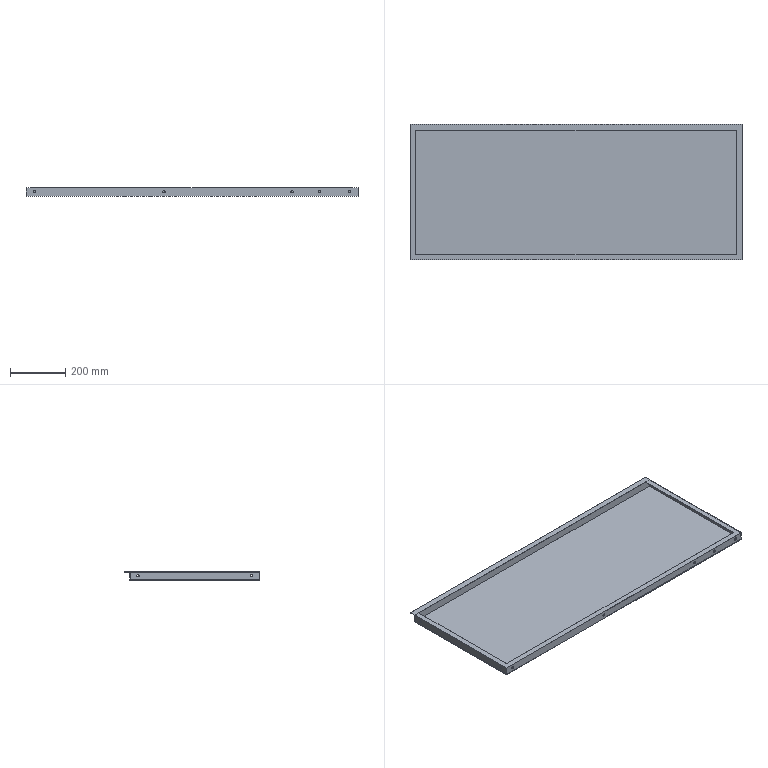Part | SolidWorks | features ICE 3, Extrusion 1, Shell 1 | 1 solid | 35 faces | box 1204 x 492 x 30 mm | volume 1446455 mm3 | cylinder 18 | plane 17 | commonest cylinder face diameters 9 x18
STEP:
#1=CARTESIAN_POINT('',(500.,0.,11.5));
#2=VERTEX_POINT('',#1);
#3=CARTESIAN_POINT('',(500.,0.,20.5));
#4=VERTEX_POINT('',#3);
#5=CARTESIAN_POINT('',(500.,0.,16.));
#6=DIRECTION('',(0.,1.,0.));
#7=DIRECTION('',(0.,0.,1.));
#8=AXIS2_PLACEMENT_3D('',#5,#6,#7);
#9=CIRCLE('',#8,4.5);
#10=EDGE_CURVE('',#2,#4,#9,.T.);
#11=ORIENTED_EDGE('',*,*,#10,.F.);
#12=CARTESIAN_POINT('',(500.,2.,11.5));
#13=VERTEX_POINT('',#12);
#14=CARTESIAN_POINT('',(500.,-43.,11.5));
#15=DIRECTION('',(0.,1.,0.));
#16=VECTOR('',#15,1000.);
#17=LINE('',#14,#16);
#18=EDGE_CURVE('',#2,#13,#17,.T.);
#19=ORIENTED_EDGE('',*,*,#18,.T.);
#20=CARTESIAN_POINT('',(500.,2.,20.5));
#21=VERTEX_POINT('',#20);
#22=CARTESIAN_POINT('',(500.,2.,16.));
#23=DIRECTION('',(0.,1.,0.));
#24=DIRECTION('',(0.,0.,1.));
#25=AXIS2_PLACEMENT_3D('',#22,#23,#24);
#26=CIRCLE('',#25,4.5);
#27=EDGE_CURVE('',#13,#21,#26,.T.);
#28=ORIENTED_EDGE('',*,*,#27,.T.);
#29=CARTESIAN_POINT('',(500.,-43.,20.5));
#30=DIRECTION('',(0.,1.,0.));
#31=VECTOR('',#30,1000.);
#32=LINE('',#29,#31);
#33=EDGE_CURVE('',#4,#21,#32,.T.);
#34=ORIENTED_EDGE('',*,*,#33,.F.);
#35=EDGE_LOOP('',(#11,#19,#28,#34));
#36=FACE_OUTER_BOUND('',#35,.T.);
#37=CARTESIAN_POINT('',(500.,-43.,16.));
#38=DIRECTION('',(0.,1.,0.));
#39=DIRECTION('',(0.,0.,1.));
#40=AXIS2_PLACEMENT_3D('',#37,#38,#39);
#41=CYLINDRICAL_SURFACE('',#40,4.5);
#42=ADVANCED_FACE('',(#36),#41,.F.);
#43=CARTESIAN_POINT('',(965.,0.,11.5));
#44=VERTEX_POINT('',#43);
#45=CARTESIAN_POINT('',(965.,0.,20.5));
#46=VERTEX_POINT('',#45);
#47=CARTESIAN_POINT('',(965.,0.,16.));
#48=DIRECTION('',(0.,1.,0.));
#49=DIRECTION('',(0.,0.,1.));
#50=AXIS2_PLACEMENT_3D('',#47,#48,#49);
#51=CIRCLE('',#50,4.5);
#52=EDGE_CURVE('',#44,#46,#51,.T.);
#53=ORIENTED_EDGE('',*,*,#52,.F.);
#54=CARTESIAN_POINT('',(965.,2.,11.5));
#55=VERTEX_POINT('',#54);
#56=CARTESIAN_POINT('',(965.,-43.,11.5));
#57=DIRECTION('',(0.,1.,0.));
#58=VECTOR('',#57,1000.);
#59=LINE('',#56,#58);
#60=EDGE_CURVE('',#44,#55,#59,.T.);
#61=ORIENTED_EDGE('',*,*,#60,.T.);
#62=CARTESIAN_POINT('',(965.,2.,20.5));
#63=VERTEX_POINT('',#62);
#64=CARTESIAN_POINT('',(965.,2.,16.));
#65=DIRECTION('',(0.,1.,0.));
#66=DIRECTION('',(0.,0.,1.));
#67=AXIS2_PLACEMENT_3D('',#64,#65,#66);
#68=CIRCLE('',#67,4.5);
#69=EDGE_CURVE('',#55,#63,#68,.T.);
#70=ORIENTED_EDGE('',*,*,#69,.T.);
#71=CARTESIAN_POINT('',(965.,-43.,20.5));
#72=DIRECTION('',(0.,1.,0.));
#73=VECTOR('',#72,1000.);
#74=LINE('',#71,#73);
#75=EDGE_CURVE('',#46,#63,#74,.T.);
#76=ORIENTED_EDGE('',*,*,#75,.F.);
#77=EDGE_LOOP('',(#53,#61,#70,#76));
#78=FACE_OUTER_BOUND('',#77,.T.);
#79=CARTESIAN_POINT('',(965.,-43.,16.));
#80=DIRECTION('',(0.,1.,0.));
#81=DIRECTION('',(0.,0.,1.));
#82=AXIS2_PLACEMENT_3D('',#79,#80,#81);
#83=CYLINDRICAL_SURFACE('',#82,4.5);
#84=ADVANCED_FACE('',(#78),#83,.F.);
#85=CARTESIAN_POINT('',(1065.,0.,11.5));
#86=VERTEX_POINT('',#85);
#87=CARTESIAN_POINT('',(1065.,0.,20.5));
#88=VERTEX_POINT('',#87);
#89=CARTESIAN_POINT('',(1065.,0.,16.));
#90=DIRECTION('',(0.,1.,0.));
#91=DIRECTION('',(0.,0.,1.));
#92=AXIS2_PLACEMENT_3D('',#89,#90,#91);
#93=CIRCLE('',#92,4.5);
#94=EDGE_CURVE('',#86,#88,#93,.T.);
#95=ORIENTED_EDGE('',*,*,#94,.F.);
#96=CARTESIAN_POINT('',(1065.,2.,11.5));
#97=VERTEX_POINT('',#96);
#98=CARTESIAN_POINT('',(1065.,-43.,11.5));
#99=DIRECTION('',(0.,1.,0.));
#100=VECTOR('',#99,1000.);
#101=LINE('',#98,#100);
#102=EDGE_CURVE('',#86,#97,#101,.T.);
#103=ORIENTED_EDGE('',*,*,#102,.T.);
#104=CARTESIAN_POINT('',(1065.,2.,20.5));
#105=VERTEX_POINT('',#104);
#106=CARTESIAN_POINT('',(1065.,2.,16.));
#107=DIRECTION('',(0.,1.,0.));
#108=DIRECTION('',(0.,0.,1.));
#109=AXIS2_PLACEMENT_3D('',#106,#107,#108);
#110=CIRCLE('',#109,4.5);
#111=EDGE_CURVE('',#97,#105,#110,.T.);
#112=ORIENTED_EDGE('',*,*,#111,.T.);
#113=CARTESIAN_POINT('',(1065.,-43.,20.5));
#114=DIRECTION('',(0.,1.,0.));
#115=VECTOR('',#114,1000.);
#116=LINE('',#113,#115);
#117=EDGE_CURVE('',#88,#105,#116,.T.);
#118=ORIENTED_EDGE('',*,*,#117,.F.);
#119=EDGE_LOOP('',(#95,#103,#112,#118));
#120=FACE_OUTER_BOUND('',#119,.T.);
#121=CARTESIAN_POINT('',(1065.,-43.,16.));
#122=DIRECTION('',(0.,1.,0.));
#123=DIRECTION('',(0.,0.,1.));
#124=AXIS2_PLACEMENT_3D('',#121,#122,#123);
#125=CYLINDRICAL_SURFACE('',#124,4.5);
#126=ADVANCED_FACE('',(#120),#125,.F.);
#127=CARTESIAN_POINT('',(30.,0.,11.5));
#128=VERTEX_POINT('',#127);
#129=CARTESIAN_POINT('',(30.,0.,20.5));
#130=VERTEX_POINT('',#129);
#131=CARTESIAN_POINT('',(30.,0.,16.));
#132=DIRECTION('',(0.,1.,0.));
#133=DIRECTION('',(0.,0.,1.));
#134=AXIS2_PLACEMENT_3D('',#131,#132,#133);
#135=CIRCLE('',#134,4.5);
#136=EDGE_CURVE('',#128,#130,#135,.T.);
#137=ORIENTED_EDGE('',*,*,#136,.F.);
#138=CARTESIAN_POINT('',(30.,2.,11.5));
#139=VERTEX_POINT('',#138);
#140=CARTESIAN_POINT('',(30.,-43.,11.5));
#141=DIRECTION('',(0.,1.,0.));
#142=VECTOR('',#141,1000.);
#143=LINE('',#140,#142);
#144=EDGE_CURVE('',#128,#139,#143,.T.);
#145=ORIENTED_EDGE('',*,*,#144,.T.);
#146=CARTESIAN_POINT('',(30.,2.,20.5));
#147=VERTEX_POINT('',#146);
#148=CARTESIAN_POINT('',(30.,2.,16.));
#149=DIRECTION('',(0.,1.,0.));
#150=DIRECTION('',(0.,0.,1.));
#151=AXIS2_PLACEMENT_3D('',#148,#149,#150);
#152=CIRCLE('',#151,4.5);
#153=EDGE_CURVE('',#139,#147,#152,.T.);
#154=ORIENTED_EDGE('',*,*,#153,.T.);
#155=CARTESIAN_POINT('',(30.,-43.,20.5));
#156=DIRECTION('',(0.,1.,0.));
#157=VECTOR('',#156,1000.);
#158=LINE('',#155,#157);
#159=EDGE_CURVE('',#130,#147,#158,.T.);
#160=ORIENTED_EDGE('',*,*,#159,.F.);
#161=EDGE_LOOP('',(#137,#145,#154,#160));
#162=FACE_OUTER_BOUND('',#161,.T.);
#163=CARTESIAN_POINT('',(30.,-43.,16.));
#164=DIRECTION('',(0.,1.,0.));
#165=DIRECTION('',(0.,0.,1.));
#166=AXIS2_PLACEMENT_3D('',#163,#164,#165);
#167=CYLINDRICAL_SURFACE('',#166,4.5);
#168=ADVANCED_FACE('',(#162),#167,.F.);
#169=CARTESIAN_POINT('',(1174.,0.,11.5));
#170=VERTEX_POINT('',#169);
#171=CARTESIAN_POINT('',(1174.,0.,20.5));
#172=VERTEX_POINT('',#171);
#173=CARTESIAN_POINT('',(1174.,0.,16.));
#174=DIRECTION('',(0.,1.,0.));
#175=DIRECTION('',(0.,0.,1.));
#176=AXIS2_PLACEMENT_3D('',#173,#174,#175);
#177=CIRCLE('',#176,4.5);
#178=EDGE_CURVE('',#170,#172,#177,.T.);
#179=ORIENTED_EDGE('',*,*,#178,.F.);
#180=CARTESIAN_POINT('',(1174.,2.,11.5));
#181=VERTEX_POINT('',#180);
#182=CARTESIAN_POINT('',(1174.,-43.,11.5));
#183=DIRECTION('',(0.,1.,0.));
#184=VECTOR('',#183,1000.);
#185=LINE('',#182,#184);
#186=EDGE_CURVE('',#170,#181,#185,.T.);
#187=ORIENTED_EDGE('',*,*,#186,.T.);
#188=CARTESIAN_POINT('',(1174.,2.,20.5));
#189=VERTEX_POINT('',#188);
#190=CARTESIAN_POINT('',(1174.,2.,16.));
#191=DIRECTION('',(0.,1.,0.));
#192=DIRECTION('',(0.,0.,1.));
#193=AXIS2_PLACEMENT_3D('',#190,#191,#192);
#194=CIRCLE('',#193,4.5);
#195=EDGE_CURVE('',#181,#189,#194,.T.);
#196=ORIENTED_EDGE('',*,*,#195,.T.);
#197=CARTESIAN_POINT('',(1174.,-43.,20.5));
#198=DIRECTION('',(0.,1.,0.));
#199=VECTOR('',#198,1000.);
#200=LINE('',#197,#199);
#201=EDGE_CURVE('',#172,#189,#200,.T.);
#202=ORIENTED_EDGE('',*,*,#201,.F.);
#203=EDGE_LOOP('',(#179,#187,#196,#202));
#204=FACE_OUTER_BOUND('',#203,.T.);
#205=CARTESIAN_POINT('',(1174.,-43.,16.));
#206=DIRECTION('',(0.,1.,0.));
#207=DIRECTION('',(0.,0.,1.));
#208=AXIS2_PLACEMENT_3D('',#205,#206,#207);
#209=CYLINDRICAL_SURFACE('',#208,4.5);
#210=ADVANCED_FACE('',(#204),#209,.F.);
#211=CARTESIAN_POINT('',(2.,30.,11.5));
#212=VERTEX_POINT('',#211);
#213=CARTESIAN_POINT('',(2.,30.,20.5));
#214=VERTEX_POINT('',#213);
#215=CARTESIAN_POINT('',(2.,30.,16.));
#216=DIRECTION('',(-1.,0.,0.));
#217=DIRECTION('',(0.,0.,-1.));
#218=AXIS2_PLACEMENT_3D('',#215,#216,#217);
#219=CIRCLE('',#218,4.5);
#220=EDGE_CURVE('',#212,#214,#219,.T.);
#221=ORIENTED_EDGE('',*,*,#220,.F.);
#222=CARTESIAN_POINT('',(0.,30.,11.5));
#223=VERTEX_POINT('',#222);
#224=CARTESIAN_POINT('',(1297.,30.,11.5));
#225=DIRECTION('',(-1.,0.,0.));
#226=VECTOR('',#225,1000.);
#227=LINE('',#224,#226);
#228=EDGE_CURVE('',#212,#223,#227,.T.);
#229=ORIENTED_EDGE('',*,*,#228,.T.);
#230=CARTESIAN_POINT('',(0.,30.,20.5));
#231=VERTEX_POINT('',#230);
#232=CARTESIAN_POINT('',(0.,30.,16.));
#233=DIRECTION('',(-1.,0.,0.));
#234=DIRECTION('',(0.,0.,-1.));
#235=AXIS2_PLACEMENT_3D('',#232,#233,#234);
#236=CIRCLE('',#235,4.5);
#237=EDGE_CURVE('',#223,#231,#236,.T.);
#238=ORIENTED_EDGE('',*,*,#237,.T.);
#239=CARTESIAN_POINT('',(1297.,30.,20.5));
#240=DIRECTION('',(-1.,0.,0.));
#241=VECTOR('',#240,1000.);
#242=LINE('',#239,#241);
#243=EDGE_CURVE('',#214,#231,#242,.T.);
#244=ORIENTED_EDGE('',*,*,#243,.F.);
#245=EDGE_LOOP('',(#221,#229,#238,#244));
#246=FACE_OUTER_BOUND('',#245,.T.);
#247=CARTESIAN_POINT('',(1297.,30.,16.));
#248=DIRECTION('',(-1.,0.,0.));
#249=DIRECTION('',(0.,0.,1.));
#250=AXIS2_PLACEMENT_3D('',#247,#248,#249);
#251=CYLINDRICAL_SURFACE('',#250,4.5);
#252=ADVANCED_FACE('',(#246),#251,.F.);
#253=CARTESIAN_POINT('',(1204.,30.,20.5));
#254=VERTEX_POINT('',#253);
#255=CARTESIAN_POINT('',(1204.,30.,11.5));
#256=VERTEX_POINT('',#255);
#257=CARTESIAN_POINT('',(1204.,30.,16.));
#258=DIRECTION('',(1.,0.,0.));
#259=DIRECTION('',(0.,0.,1.));
#260=AXIS2_PLACEMENT_3D('',#257,#258,#259);
#261=CIRCLE('',#260,4.5);
#262=EDGE_CURVE('',#254,#256,#261,.T.);
#263=ORIENTED_EDGE('',*,*,#262,.T.);
#264=CARTESIAN_POINT('',(1202.,30.,11.5));
#265=VERTEX_POINT('',#264);
#266=CARTESIAN_POINT('',(1297.,30.,11.5));
#267=DIRECTION('',(-1.,0.,0.));
#268=VECTOR('',#267,1000.);
#269=LINE('',#266,#268);
#270=EDGE_CURVE('',#256,#265,#269,.T.);
#271=ORIENTED_EDGE('',*,*,#270,.T.);
#272=CARTESIAN_POINT('',(1202.,30.,20.5));
#273=VERTEX_POINT('',#272);
#274=CARTESIAN_POINT('',(1202.,30.,16.));
#275=DIRECTION('',(1.,0.,0.));
#276=DIRECTION('',(0.,0.,1.));
#277=AXIS2_PLACEMENT_3D('',#274,#275,#276);
#278=CIRCLE('',#277,4.5);
#279=EDGE_CURVE('',#273,#265,#278,.T.);
#280=ORIENTED_EDGE('',*,*,#279,.F.);
#281=CARTESIAN_POINT('',(1297.,30.,20.5));
#282=DIRECTION('',(-1.,0.,0.));
#283=VECTOR('',#282,1000.);
#284=LINE('',#281,#283);
#285=EDGE_CURVE('',#254,#273,#284,.T.);
#286=ORIENTED_EDGE('',*,*,#285,.F.);
#287=EDGE_LOOP('',(#263,#271,#280,#286));
#288=FACE_OUTER_BOUND('',#287,.T.);
#289=CARTESIAN_POINT('',(1297.,30.,16.));
#290=DIRECTION('',(-1.,0.,0.));
#291=DIRECTION('',(0.,0.,1.));
#292=AXIS2_PLACEMENT_3D('',#289,#290,#291);
#293=CYLINDRICAL_SURFACE('',#292,4.5);
#294=ADVANCED_FACE('',(#288),#293,.F.);
#295=CARTESIAN_POINT('',(2.,442.,11.5));
#296=VERTEX_POINT('',#295);
#297=CARTESIAN_POINT('',(2.,442.,20.5));
#298=VERTEX_POINT('',#297);
#299=CARTESIAN_POINT('',(2.,442.,16.));
#300=DIRECTION('',(-1.,0.,0.));
#301=DIRECTION('',(0.,0.,-1.));
#302=AXIS2_PLACEMENT_3D('',#299,#300,#301);
#303=CIRCLE('',#302,4.5);
#304=EDGE_CURVE('',#296,#298,#303,.T.);
#305=ORIENTED_EDGE('',*,*,#304,.F.);
#306=CARTESIAN_POINT('',(0.,442.,11.5));
#307=VERTEX_POINT('',#306);
#308=CARTESIAN_POINT('',(1297.,442.,11.5));
#309=DIRECTION('',(-1.,0.,0.));
#310=VECTOR('',#309,1000.);
#311=LINE('',#308,#310);
#312=EDGE_CURVE('',#296,#307,#311,.T.);
#313=ORIENTED_EDGE('',*,*,#312,.T.);
#314=CARTESIAN_POINT('',(0.,442.,20.5));
#315=VERTEX_POINT('',#314);
#316=CARTESIAN_POINT('',(0.,442.,16.));
#317=DIRECTION('',(-1.,0.,0.));
#318=DIRECTION('',(0.,0.,-1.));
#319=AXIS2_PLACEMENT_3D('',#316,#317,#318);
#320=CIRCLE('',#319,4.5);
#321=EDGE_CURVE('',#307,#315,#320,.T.);
#322=ORIENTED_EDGE('',*,*,#321,.T.);
#323=CARTESIAN_POINT('',(1297.,442.,20.5));
#324=DIRECTION('',(-1.,0.,0.));
#325=VECTOR('',#324,1000.);
#326=LINE('',#323,#325);
#327=EDGE_CURVE('',#298,#315,#326,.T.);
#328=ORIENTED_EDGE('',*,*,#327,.F.);
#329=EDGE_LOOP('',(#305,#313,#322,#328));
#330=FACE_OUTER_BOUND('',#329,.T.);
#331=CARTESIAN_POINT('',(1297.,442.,16.));
#332=DIRECTION('',(-1.,0.,0.));
#333=DIRECTION('',(0.,0.,1.));
#334=AXIS2_PLACEMENT_3D('',#331,#332,#333);
#335=CYLINDRICAL_SURFACE('',#334,4.5);
#336=ADVANCED_FACE('',(#330),#335,.F.);
#337=CARTESIAN_POINT('',(1204.,442.,20.5));
#338=VERTEX_POINT('',#337);
#339=CARTESIAN_POINT('',(1204.,442.,11.5));
#340=VERTEX_POINT('',#339);
#341=CARTESIAN_POINT('',(1204.,442.,16.));
#342=DIRECTION('',(1.,0.,0.));
#343=DIRECTION('',(0.,0.,1.));
#344=AXIS2_PLACEMENT_3D('',#341,#342,#343);
#345=CIRCLE('',#344,4.5);
#346=EDGE_CURVE('',#338,#340,#345,.T.);
#347=ORIENTED_EDGE('',*,*,#346,.T.);
#348=CARTESIAN_POINT('',(1202.,442.,11.5));
#349=VERTEX_POINT('',#348);
#350=CARTESIAN_POINT('',(1297.,442.,11.5));
#351=DIRECTION('',(-1.,0.,0.));
#352=VECTOR('',#351,1000.);
#353=LINE('',#350,#352);
#354=EDGE_CURVE('',#340,#349,#353,.T.);
#355=ORIENTED_EDGE('',*,*,#354,.T.);
#356=CARTESIAN_POINT('',(1202.,442.,20.5));
#357=VERTEX_POINT('',#356);
#358=CARTESIAN_POINT('',(1202.,442.,16.));
#359=DIRECTION('',(1.,0.,0.));
#360=DIRECTION('',(0.,0.,1.));
#361=AXIS2_PLACEMENT_3D('',#358,#359,#360);
#362=CIRCLE('',#361,4.5);
#363=EDGE_CURVE('',#357,#349,#362,.T.);
#364=ORIENTED_EDGE('',*,*,#363,.F.);
#365=CARTESIAN_POINT('',(1297.,442.,20.5));
#366=DIRECTION('',(-1.,0.,0.));
#367=VECTOR('',#366,1000.);
#368=LINE('',#365,#367);
#369=EDGE_CURVE('',#338,#357,#368,.T.);
#370=ORIENTED_EDGE('',*,*,#369,.F.);
#371=EDGE_LOOP('',(#347,#355,#364,#370));
#372=FACE_OUTER_BOUND('',#371,.T.);
#373=CARTESIAN_POINT('',(1297.,442.,16.));
#374=DIRECTION('',(-1.,0.,0.));
#375=DIRECTION('',(0.,0.,1.));
#376=AXIS2_PLACEMENT_3D('',#373,#374,#375);
#377=CYLINDRICAL_SURFACE('',#376,4.5);
#378=ADVANCED_FACE('',(#372),#377,.F.);
#379=CARTESIAN_POINT('',(2.,442.,16.));
#380=DIRECTION('',(-1.,0.,0.));
#381=DIRECTION('',(0.,0.,-1.));
#382=AXIS2_PLACEMENT_3D('',#379,#380,#381);
#383=CIRCLE('',#382,4.5);
#384=EDGE_CURVE('',#298,#296,#383,.T.);
#385=ORIENTED_EDGE('',*,*,#384,.T.);
#386=ORIENTED_EDGE('',*,*,#304,.T.);
#387=EDGE_LOOP('',(#385,#386));
#388=FACE_BOUND('',#387,.T.);
#389=CARTESIAN_POINT('',(2.,470.,28.));
#390=VERTEX_POINT('',#389);
#391=CARTESIAN_POINT('',(2.,470.,2.));
#392=VERTEX_POINT('',#391);
#393=CARTESIAN_POINT('',(2.,470.,30.));
#394=DIRECTION('',(0.,0.,-1.));
#395=VECTOR('',#394,1000.);
#396=LINE('',#393,#395);
#397=EDGE_CURVE('',#390,#392,#396,.T.);
#398=ORIENTED_EDGE('',*,*,#397,.F.);
#399=CARTESIAN_POINT('',(2.,2.,28.));
#400=VERTEX_POINT('',#399);
#401=CARTESIAN_POINT('',(2.,0.,28.));
#402=DIRECTION('',(0.,-1.,0.));
#403=VECTOR('',#402,1000.);
#404=LINE('',#401,#403);
#405=EDGE_CURVE('',#390,#400,#404,.T.);
#406=ORIENTED_EDGE('',*,*,#405,.T.);
#407=CARTESIAN_POINT('',(2.,2.,2.));
#408=VERTEX_POINT('',#407);
#409=CARTESIAN_POINT('',(2.,2.,30.));
#410=DIRECTION('',(0.,0.,-1.));
#411=VECTOR('',#410,1000.);
#412=LINE('',#409,#411);
#413=EDGE_CURVE('',#400,#408,#412,.T.);
#414=ORIENTED_EDGE('',*,*,#413,.T.);
#415=CARTESIAN_POINT('',(2.,472.,2.));
#416=DIRECTION('',(0.,-1.,0.));
#417=VECTOR('',#416,1000.);
#418=LINE('',#415,#417);
#419=EDGE_CURVE('',#392,#408,#418,.T.);
#420=ORIENTED_EDGE('',*,*,#419,.F.);
#421=EDGE_LOOP('',(#398,#406,#414,#420));
#422=FACE_OUTER_BOUND('',#421,.T.);
#423=CARTESIAN_POINT('',(2.,30.,16.));
#424=DIRECTION('',(-1.,0.,0.));
#425=DIRECTION('',(0.,0.,-1.));
#426=AXIS2_PLACEMENT_3D('',#423,#424,#425);
#427=CIRCLE('',#426,4.5);
#428=EDGE_CURVE('',#214,#212,#427,.T.);
#429=ORIENTED_EDGE('',*,*,#428,.T.);
#430=ORIENTED_EDGE('',*,*,#220,.T.);
#431=EDGE_LOOP('',(#429,#430));
#432=FACE_BOUND('',#431,.T.);
#433=CARTESIAN_POINT('',(2.,0.,30.));
#434=DIRECTION('',(1.,0.,0.));
#435=DIRECTION('',(0.,0.,-1.));
#436=AXIS2_PLACEMENT_3D('',#433,#434,#435);
#437=PLANE('',#436);
#438=ADVANCED_FACE('',(#388,#422,#432),#437,.T.);
#439=ORIENTED_EDGE('',*,*,#363,.T.);
#440=CARTESIAN_POINT('',(1202.,442.,16.));
#441=DIRECTION('',(1.,0.,0.));
#442=DIRECTION('',(0.,0.,1.));
#443=AXIS2_PLACEMENT_3D('',#440,#441,#442);
#444=CIRCLE('',#443,4.5);
#445=EDGE_CURVE('',#349,#357,#444,.T.);
#446=ORIENTED_EDGE('',*,*,#445,.T.);
#447=EDGE_LOOP('',(#439,#446));
#448=FACE_BOUND('',#447,.T.);
#449=CARTESIAN_POINT('',(1202.,2.,28.));
#450=VERTEX_POINT('',#449);
#451=CARTESIAN_POINT('',(1202.,2.,2.));
#452=VERTEX_POINT('',#451);
#453=CARTESIAN_POINT('',(1202.,2.,30.));
#454=DIRECTION('',(0.,0.,-1.));
#455=VECTOR('',#454,1000.);
#456=LINE('',#453,#455);
#457=EDGE_CURVE('',#450,#452,#456,.T.);
#458=ORIENTED_EDGE('',*,*,#457,.F.);
#459=CARTESIAN_POINT('',(1202.,470.,28.));
#460=VERTEX_POINT('',#459);
#461=CARTESIAN_POINT('',(1202.,0.,28.));
#462=DIRECTION('',(0.,1.,0.));
#463=VECTOR('',#462,1000.);
#464=LINE('',#461,#463);
#465=EDGE_CURVE('',#450,#460,#464,.T.);
#466=ORIENTED_EDGE('',*,*,#465,.T.);
#467=CARTESIAN_POINT('',(1202.,470.,2.));
#468=VERTEX_POINT('',#467);
#469=CARTESIAN_POINT('',(1202.,470.,30.));
#470=DIRECTION('',(0.,0.,-1.));
#471=VECTOR('',#470,1000.);
#472=LINE('',#469,#471);
#473=EDGE_CURVE('',#460,#468,#472,.T.);
#474=ORIENTED_EDGE('',*,*,#473,.T.);
#475=CARTESIAN_POINT('',(1202.,472.,2.));
#476=DIRECTION('',(0.,1.,0.));
#477=VECTOR('',#476,1000.);
#478=LINE('',#475,#477);
#479=EDGE_CURVE('',#452,#468,#478,.T.);
#480=ORIENTED_EDGE('',*,*,#479,.F.);
#481=EDGE_LOOP('',(#458,#466,#474,#480));
#482=FACE_OUTER_BOUND('',#481,.T.);
#483=ORIENTED_EDGE('',*,*,#279,.T.);
#484=CARTESIAN_POINT('',(1202.,30.,16.));
#485=DIRECTION('',(1.,0.,0.));
#486=DIRECTION('',(0.,0.,1.));
#487=AXIS2_PLACEMENT_3D('',#484,#485,#486);
#488=CIRCLE('',#487,4.5);
#489=EDGE_CURVE('',#265,#273,#488,.T.);
#490=ORIENTED_EDGE('',*,*,#489,.T.);
#491=EDGE_LOOP('',(#483,#490));
#492=FACE_BOUND('',#491,.T.);
#493=CARTESIAN_POINT('',(1202.,0.,30.));
#494=DIRECTION('',(-1.,0.,0.));
#495=DIRECTION('',(0.,0.,1.));
#496=AXIS2_PLACEMENT_3D('',#493,#494,#495);
#497=PLANE('',#496);
#498=ADVANCED_FACE('',(#448,#482,#492),#497,.T.);
#499=CARTESIAN_POINT('',(0.,442.,16.));
#500=DIRECTION('',(-1.,0.,0.));
#501=DIRECTION('',(0.,0.,-1.));
#502=AXIS2_PLACEMENT_3D('',#499,#500,#501);
#503=CIRCLE('',#502,4.5);
#504=EDGE_CURVE('',#315,#307,#503,.T.);
#505=ORIENTED_EDGE('',*,*,#504,.F.);
#506=ORIENTED_EDGE('',*,*,#321,.F.);
#507=EDGE_LOOP('',(#505,#506));
#508=FACE_BOUND('',#507,.T.);
#509=CARTESIAN_POINT('',(0.,492.,30.));
#510=VERTEX_POINT('',#509);
#511=CARTESIAN_POINT('',(0.,0.,30.));
#512=VERTEX_POINT('',#511);
#513=CARTESIAN_POINT('',(0.,0.,30.));
#514=DIRECTION('',(0.,-1.,0.));
#515=VECTOR('',#514,1000.);
#516=LINE('',#513,#515);
#517=EDGE_CURVE('',#510,#512,#516,.T.);
#518=ORIENTED_EDGE('',*,*,#517,.F.);
#519=CARTESIAN_POINT('',(0.,492.,28.));
#520=VERTEX_POINT('',#519);
#521=CARTESIAN_POINT('',(0.,492.,28.));
#522=DIRECTION('',(0.,0.,1.));
#523=VECTOR('',#522,1000.);
#524=LINE('',#521,#523);
#525=EDGE_CURVE('',#520,#510,#524,.T.);
#526=ORIENTED_EDGE('',*,*,#525,.F.);
#527=CARTESIAN_POINT('',(0.,472.,28.));
#528=VERTEX_POINT('',#527);
#529=CARTESIAN_POINT('',(0.,492.,28.));
#530=DIRECTION('',(0.,-1.,0.));
#531=VECTOR('',#530,1000.);
#532=LINE('',#529,#531);
#533=EDGE_CURVE('',#520,#528,#532,.T.);
#534=ORIENTED_EDGE('',*,*,#533,.T.);
#535=CARTESIAN_POINT('',(0.,472.,0.));
#536=VERTEX_POINT('',#535);
#537=CARTESIAN_POINT('',(0.,472.,30.));
#538=DIRECTION('',(0.,0.,-1.));
#539=VECTOR('',#538,1000.);
#540=LINE('',#537,#539);
#541=EDGE_CURVE('',#528,#536,#540,.T.);
#542=ORIENTED_EDGE('',*,*,#541,.T.);
#543=CARTESIAN_POINT('',(0.,0.,0.));
#544=VERTEX_POINT('',#543);
#545=CARTESIAN_POINT('',(0.,0.,0.));
#546=DIRECTION('',(0.,-1.,0.));
#547=VECTOR('',#546,1000.);
#548=LINE('',#545,#547);
#549=EDGE_CURVE('',#536,#544,#548,.T.);
#550=ORIENTED_EDGE('',*,*,#549,.T.);
#551=CARTESIAN_POINT('',(0.,0.,30.));
#552=DIRECTION('',(0.,0.,-1.));
#553=VECTOR('',#552,1000.);
#554=LINE('',#551,#553);
#555=EDGE_CURVE('',#512,#544,#554,.T.);
#556=ORIENTED_EDGE('',*,*,#555,.F.);
#557=EDGE_LOOP('',(#518,#526,#534,#542,#550,#556));
#558=FACE_OUTER_BOUND('',#557,.T.);
#559=CARTESIAN_POINT('',(0.,30.,16.));
#560=DIRECTION('',(-1.,0.,0.));
#561=DIRECTION('',(0.,0.,-1.));
#562=AXIS2_PLACEMENT_3D('',#559,#560,#561);
#563=CIRCLE('',#562,4.5);
#564=EDGE_CURVE('',#231,#223,#563,.T.);
#565=ORIENTED_EDGE('',*,*,#564,.F.);
#566=ORIENTED_EDGE('',*,*,#237,.F.);
#567=EDGE_LOOP('',(#565,#566));
#568=FACE_BOUND('',#567,.T.);
#569=CARTESIAN_POINT('',(0.,0.,30.));
#570=DIRECTION('',(1.,0.,0.));
#571=DIRECTION('',(0.,0.,-1.));
#572=AXIS2_PLACEMENT_3D('',#569,#570,#571);
#573=PLANE('',#572);
#574=ADVANCED_FACE('',(#508,#558,#568),#573,.F.);
#575=ORIENTED_EDGE('',*,*,#346,.F.);
#576=CARTESIAN_POINT('',(1204.,442.,16.));
#577=DIRECTION('',(1.,0.,0.));
#578=DIRECTION('',(0.,0.,1.));
#579=AXIS2_PLACEMENT_3D('',#576,#577,#578);
#580=CIRCLE('',#579,4.5);
#581=EDGE_CURVE('',#340,#338,#580,.T.);
#582=ORIENTED_EDGE('',*,*,#581,.F.);
#583=EDGE_LOOP('',(#575,#582));
#584=FACE_BOUND('',#583,.T.);
#585=CARTESIAN_POINT('',(1204.,0.,30.));
#586=VERTEX_POINT('',#585);
#587=CARTESIAN_POINT('',(1204.,0.,0.));
#588=VERTEX_POINT('',#587);
#589=CARTESIAN_POINT('',(1204.,0.,30.));
#590=DIRECTION('',(0.,0.,-1.));
#591=VECTOR('',#590,1000.);
#592=LINE('',#589,#591);
#593=EDGE_CURVE('',#586,#588,#592,.T.);
#594=ORIENTED_EDGE('',*,*,#593,.T.);
#595=CARTESIAN_POINT('',(1204.,472.,0.));
#596=VERTEX_POINT('',#595);
#597=CARTESIAN_POINT('',(1204.,0.,0.));
#598=DIRECTION('',(0.,1.,0.));
#599=VECTOR('',#598,1000.);
#600=LINE('',#597,#599);
#601=EDGE_CURVE('',#588,#596,#600,.T.);
#602=ORIENTED_EDGE('',*,*,#601,.T.);
#603=CARTESIAN_POINT('',(1204.,472.,28.));
#604=VERTEX_POINT('',#603);
#605=CARTESIAN_POINT('',(1204.,472.,30.));
#606=DIRECTION('',(0.,0.,-1.));
#607=VECTOR('',#606,1000.);
#608=LINE('',#605,#607);
#609=EDGE_CURVE('',#604,#596,#608,.T.);
#610=ORIENTED_EDGE('',*,*,#609,.F.);
#611=CARTESIAN_POINT('',(1204.,492.,28.));
#612=VERTEX_POINT('',#611);
#613=CARTESIAN_POINT('',(1204.,492.,28.));
#614=DIRECTION('',(0.,1.,0.));
#615=VECTOR('',#614,1000.);
#616=LINE('',#613,#615);
#617=EDGE_CURVE('',#604,#612,#616,.T.);
#618=ORIENTED_EDGE('',*,*,#617,.T.);
#619=CARTESIAN_POINT('',(1204.,492.,30.));
#620=VERTEX_POINT('',#619);
#621=CARTESIAN_POINT('',(1204.,492.,28.));
#622=DIRECTION('',(0.,0.,1.));
#623=VECTOR('',#622,1000.);
#624=LINE('',#621,#623);
#625=EDGE_CURVE('',#612,#620,#624,.T.);
#626=ORIENTED_EDGE('',*,*,#625,.T.);
#627=CARTESIAN_POINT('',(1204.,0.,30.));
#628=DIRECTION('',(0.,1.,0.));
#629=VECTOR('',#628,1000.);
#630=LINE('',#627,#629);
#631=EDGE_CURVE('',#586,#620,#630,.T.);
#632=ORIENTED_EDGE('',*,*,#631,.F.);
#633=EDGE_LOOP('',(#594,#602,#610,#618,#626,#632));
#634=FACE_OUTER_BOUND('',#633,.T.);
#635=ORIENTED_EDGE('',*,*,#262,.F.);
#636=CARTESIAN_POINT('',(1204.,30.,16.));
#637=DIRECTION('',(1.,0.,0.));
#638=DIRECTION('',(0.,0.,1.));
#639=AXIS2_PLACEMENT_3D('',#636,#637,#638);
#640=CIRCLE('',#639,4.5);
#641=EDGE_CURVE('',#256,#254,#640,.T.);
#642=ORIENTED_EDGE('',*,*,#641,.F.);
#643=EDGE_LOOP('',(#635,#642));
#644=FACE_BOUND('',#643,.T.);
#645=CARTESIAN_POINT('',(1204.,0.,30.));
#646=DIRECTION('',(-1.,0.,0.));
#647=DIRECTION('',(0.,0.,1.));
#648=AXIS2_PLACEMENT_3D('',#645,#646,#647);
#649=PLANE('',#648);
#650=ADVANCED_FACE('',(#584,#634,#644),#649,.F.);
#651=CARTESIAN_POINT('',(0.,472.,28.));
#652=DIRECTION('',(-1.,0.,0.));
#653=VECTOR('',#652,1000.);
#654=LINE('',#651,#653);
#655=EDGE_CURVE('',#604,#528,#654,.T.);
#656=ORIENTED_EDGE('',*,*,#655,.F.);
#657=ORIENTED_EDGE('',*,*,#609,.T.);
#658=CARTESIAN_POINT('',(0.,472.,0.));
#659=DIRECTION('',(-1.,0.,0.));
#660=VECTOR('',#659,1000.);
#661=LINE('',#658,#660);
#662=EDGE_CURVE('',#596,#536,#661,.T.);
#663=ORIENTED_EDGE('',*,*,#662,.T.);
#664=ORIENTED_EDGE('',*,*,#541,.F.);
#665=EDGE_LOOP('',(#656,#657,#663,#664));
#666=FACE_OUTER_BOUND('',#665,.T.);
#667=CARTESIAN_POINT('',(0.,472.,30.));
#668=DIRECTION('',(0.,-1.,0.));
#669=DIRECTION('',(0.,0.,-1.));
#670=AXIS2_PLACEMENT_3D('',#667,#668,#669);
#671=PLANE('',#670);
#672=ADVANCED_FACE('',(#666),#671,.F.);
#673=CARTESIAN_POINT('',(500.,2.,16.));
#674=DIRECTION('',(0.,1.,0.));
#675=DIRECTION('',(0.,0.,1.));
#676=AXIS2_PLACEMENT_3D('',#673,#674,#675);
#677=CIRCLE('',#676,4.5);
#678=EDGE_CURVE('',#21,#13,#677,.T.);
#679=ORIENTED_EDGE('',*,*,#678,.F.);
#680=ORIENTED_EDGE('',*,*,#27,.F.);
#681=EDGE_LOOP('',(#679,#680));
#682=FACE_BOUND('',#681,.T.);
#683=CARTESIAN_POINT('',(965.,2.,16.));
#684=DIRECTION('',(0.,1.,0.));
#685=DIRECTION('',(0.,0.,1.));
#686=AXIS2_PLACEMENT_3D('',#683,#684,#685);
#687=CIRCLE('',#686,4.5);
#688=EDGE_CURVE('',#63,#55,#687,.T.);
#689=ORIENTED_EDGE('',*,*,#688,.F.);
#690=ORIENTED_EDGE('',*,*,#69,.F.);
#691=EDGE_LOOP('',(#689,#690));
#692=FACE_BOUND('',#691,.T.);
#693=CARTESIAN_POINT('',(1065.,2.,16.));
#694=DIRECTION('',(0.,1.,0.));
#695=DIRECTION('',(0.,0.,1.));
#696=AXIS2_PLACEMENT_3D('',#693,#694,#695);
#697=CIRCLE('',#696,4.5);
#698=EDGE_CURVE('',#105,#97,#697,.T.);
#699=ORIENTED_EDGE('',*,*,#698,.F.);
#700=ORIENTED_EDGE('',*,*,#111,.F.);
#701=EDGE_LOOP('',(#699,#700));
#702=FACE_BOUND('',#701,.T.);
#703=CARTESIAN_POINT('',(30.,2.,16.));
#704=DIRECTION('',(0.,1.,0.));
#705=DIRECTION('',(0.,0.,1.));
#706=AXIS2_PLACEMENT_3D('',#703,#704,#705);
#707=CIRCLE('',#706,4.5);
#708=EDGE_CURVE('',#147,#139,#707,.T.);
#709=ORIENTED_EDGE('',*,*,#708,.F.);
#710=ORIENTED_EDGE('',*,*,#153,.F.);
#711=EDGE_LOOP('',(#709,#710));
#712=FACE_BOUND('',#711,.T.);
#713=CARTESIAN_POINT('',(1174.,2.,16.));
#714=DIRECTION('',(0.,1.,0.));
#715=DIRECTION('',(0.,0.,1.));
#716=AXIS2_PLACEMENT_3D('',#713,#714,#715);
#717=CIRCLE('',#716,4.5);
#718=EDGE_CURVE('',#189,#181,#717,.T.);
#719=ORIENTED_EDGE('',*,*,#718,.F.);
#720=ORIENTED_EDGE('',*,*,#195,.F.);
#721=EDGE_LOOP('',(#719,#720));
#722=FACE_BOUND('',#721,.T.);
#723=ORIENTED_EDGE('',*,*,#413,.F.);
#724=CARTESIAN_POINT('',(0.,2.,28.));
#725=DIRECTION('',(1.,0.,0.));
#726=VECTOR('',#725,1000.);
#727=LINE('',#724,#726);
#728=EDGE_CURVE('',#400,#450,#727,.T.);
#729=ORIENTED_EDGE('',*,*,#728,.T.);
#730=ORIENTED_EDGE('',*,*,#457,.T.);
#731=CARTESIAN_POINT('',(0.,2.,2.));
#732=DIRECTION('',(1.,0.,0.));
#733=VECTOR('',#732,1000.);
#734=LINE('',#731,#733);
#735=EDGE_CURVE('',#408,#452,#734,.T.);
#736=ORIENTED_EDGE('',*,*,#735,.F.);
#737=EDGE_LOOP('',(#723,#729,#730,#736));
#738=FACE_OUTER_BOUND('',#737,.T.);
#739=CARTESIAN_POINT('',(0.,2.,30.));
#740=DIRECTION('',(0.,1.,0.));
#741=DIRECTION('',(0.,0.,1.));
#742=AXIS2_PLACEMENT_3D('',#739,#740,#741);
#743=PLANE('',#742);
#744=ADVANCED_FACE('',(#682,#692,#702,#712,#722,#738),#743,.T.);
#745=CARTESIAN_POINT('',(1184.,470.,30.));
#746=VERTEX_POINT('',#745);
#747=CARTESIAN_POINT('',(20.,470.,30.));
#748=VERTEX_POINT('',#747);
#749=CARTESIAN_POINT('',(0.,470.,30.));
#750=DIRECTION('',(-1.,0.,0.));
#751=VECTOR('',#750,1000.);
#752=LINE('',#749,#751);
#753=EDGE_CURVE('',#746,#748,#752,.T.);
#754=ORIENTED_EDGE('',*,*,#753,.T.);
#755=CARTESIAN_POINT('',(20.,470.,28.));
#756=VERTEX_POINT('',#755);
#757=CARTESIAN_POINT('',(20.,470.,28.));
#758=DIRECTION('',(0.,0.,1.));
#759=VECTOR('',#758,1000.);
#760=LINE('',#757,#759);
#761=EDGE_CURVE('',#756,#748,#760,.T.);
#762=ORIENTED_EDGE('',*,*,#761,.F.);
#763=CARTESIAN_POINT('',(0.,470.,28.));
#764=DIRECTION('',(-1.,0.,0.));
#765=VECTOR('',#764,1000.);
#766=LINE('',#763,#765);
#767=EDGE_CURVE('',#756,#390,#766,.T.);
#768=ORIENTED_EDGE('',*,*,#767,.T.);
#769=ORIENTED_EDGE('',*,*,#397,.T.);
#770=CARTESIAN_POINT('',(0.,470.,2.));
#771=DIRECTION('',(-1.,0.,0.));
#772=VECTOR('',#771,1000.);
#773=LINE('',#770,#772);
#774=EDGE_CURVE('',#468,#392,#773,.T.);
#775=ORIENTED_EDGE('',*,*,#774,.F.);
#776=ORIENTED_EDGE('',*,*,#473,.F.);
#777=CARTESIAN_POINT('',(1184.,470.,28.));
#778=VERTEX_POINT('',#777);
#779=CARTESIAN_POINT('',(0.,470.,28.));
#780=DIRECTION('',(-1.,0.,0.));
#781=VECTOR('',#780,1000.);
#782=LINE('',#779,#781);
#783=EDGE_CURVE('',#460,#778,#782,.T.);
#784=ORIENTED_EDGE('',*,*,#783,.T.);
#785=CARTESIAN_POINT('',(1184.,470.,28.));
#786=DIRECTION('',(0.,0.,1.));
#787=VECTOR('',#786,1000.);
#788=LINE('',#785,#787);
#789=EDGE_CURVE('',#778,#746,#788,.T.);
#790=ORIENTED_EDGE('',*,*,#789,.T.);
#791=EDGE_LOOP('',(#754,#762,#768,#769,#775,#776,#784,#790));
#792=FACE_OUTER_BOUND('',#791,.T.);
#793=CARTESIAN_POINT('',(0.,470.,30.));
#794=DIRECTION('',(0.,-1.,0.));
#795=DIRECTION('',(0.,0.,-1.));
#796=AXIS2_PLACEMENT_3D('',#793,#794,#795);
#797=PLANE('',#796);
#798=ADVANCED_FACE('',(#792),#797,.T.);
#799=ORIENTED_EDGE('',*,*,#753,.F.);
#800=CARTESIAN_POINT('',(1184.,20.,30.));
#801=VERTEX_POINT('',#800);
#802=CARTESIAN_POINT('',(1184.,20.,30.));
#803=DIRECTION('',(0.,1.,0.));
#804=VECTOR('',#803,1000.);
#805=LINE('',#802,#804);
#806=EDGE_CURVE('',#801,#746,#805,.T.);
#807=ORIENTED_EDGE('',*,*,#806,.F.);
#808=CARTESIAN_POINT('',(20.,20.,30.));
#809=VERTEX_POINT('',#808);
#810=CARTESIAN_POINT('',(20.,20.,30.));
#811=DIRECTION('',(1.,0.,0.));
#812=VECTOR('',#811,1000.);
#813=LINE('',#810,#812);
#814=EDGE_CURVE('',#809,#801,#813,.T.);
#815=ORIENTED_EDGE('',*,*,#814,.F.);
#816=CARTESIAN_POINT('',(20.,20.,30.));
#817=DIRECTION('',(0.,-1.,0.));
#818=VECTOR('',#817,1000.);
#819=LINE('',#816,#818);
#820=EDGE_CURVE('',#748,#809,#819,.T.);
#821=ORIENTED_EDGE('',*,*,#820,.F.);
#822=EDGE_LOOP('',(#799,#807,#815,#821));
#823=FACE_BOUND('',#822,.T.);
#824=ORIENTED_EDGE('',*,*,#517,.T.);
#825=CARTESIAN_POINT('',(0.,0.,30.));
#826=DIRECTION('',(1.,0.,0.));
#827=VECTOR('',#826,1000.);
#828=LINE('',#825,#827);
#829=EDGE_CURVE('',#512,#586,#828,.T.);
#830=ORIENTED_EDGE('',*,*,#829,.T.);
#831=ORIENTED_EDGE('',*,*,#631,.T.);
#832=CARTESIAN_POINT('',(0.,492.,30.));
#833=DIRECTION('',(-1.,0.,0.));
#834=VECTOR('',#833,1000.);
#835=LINE('',#832,#834);
#836=EDGE_CURVE('',#620,#510,#835,.T.);
#837=ORIENTED_EDGE('',*,*,#836,.T.);
#838=EDGE_LOOP('',(#824,#830,#831,#837));
#839=FACE_OUTER_BOUND('',#838,.T.);
#840=CARTESIAN_POINT('',(0.,472.,30.));
#841=DIRECTION('',(0.,0.,-1.));
#842=DIRECTION('',(-1.,0.,0.));
#843=AXIS2_PLACEMENT_3D('',#840,#841,#842);
#844=PLANE('',#843);
#845=ADVANCED_FACE('',(#823,#839),#844,.F.);
#846=CARTESIAN_POINT('',(500.,0.,16.));
#847=DIRECTION('',(0.,1.,0.));
#848=DIRECTION('',(0.,0.,1.));
#849=AXIS2_PLACEMENT_3D('',#846,#847,#848);
#850=CIRCLE('',#849,4.5);
#851=EDGE_CURVE('',#4,#2,#850,.T.);
#852=ORIENTED_EDGE('',*,*,#851,.T.);
#853=ORIENTED_EDGE('',*,*,#10,.T.);
#854=EDGE_LOOP('',(#852,#853));
#855=FACE_BOUND('',#854,.T.);
#856=CARTESIAN_POINT('',(965.,0.,16.));
#857=DIRECTION('',(0.,1.,0.));
#858=DIRECTION('',(0.,0.,1.));
#859=AXIS2_PLACEMENT_3D('',#856,#857,#858);
#860=CIRCLE('',#859,4.5);
#861=EDGE_CURVE('',#46,#44,#860,.T.);
#862=ORIENTED_EDGE('',*,*,#861,.T.);
#863=ORIENTED_EDGE('',*,*,#52,.T.);
#864=EDGE_LOOP('',(#862,#863));
#865=FACE_BOUND('',#864,.T.);
#866=CARTESIAN_POINT('',(1065.,0.,16.));
#867=DIRECTION('',(0.,1.,0.));
#868=DIRECTION('',(0.,0.,1.));
#869=AXIS2_PLACEMENT_3D('',#866,#867,#868);
#870=CIRCLE('',#869,4.5);
#871=EDGE_CURVE('',#88,#86,#870,.T.);
#872=ORIENTED_EDGE('',*,*,#871,.T.);
#873=ORIENTED_EDGE('',*,*,#94,.T.);
#874=EDGE_LOOP('',(#872,#873));
#875=FACE_BOUND('',#874,.T.);
#876=CARTESIAN_POINT('',(30.,0.,16.));
#877=DIRECTION('',(0.,1.,0.));
#878=DIRECTION('',(0.,0.,1.));
#879=AXIS2_PLACEMENT_3D('',#876,#877,#878);
#880=CIRCLE('',#879,4.5);
#881=EDGE_CURVE('',#130,#128,#880,.T.);
#882=ORIENTED_EDGE('',*,*,#881,.T.);
#883=ORIENTED_EDGE('',*,*,#136,.T.);
#884=EDGE_LOOP('',(#882,#883));
#885=FACE_BOUND('',#884,.T.);
#886=CARTESIAN_POINT('',(1174.,0.,16.));
#887=DIRECTION('',(0.,1.,0.));
#888=DIRECTION('',(0.,0.,1.));
#889=AXIS2_PLACEMENT_3D('',#886,#887,#888);
#890=CIRCLE('',#889,4.5);
#891=EDGE_CURVE('',#172,#170,#890,.T.);
#892=ORIENTED_EDGE('',*,*,#891,.T.);
#893=ORIENTED_EDGE('',*,*,#178,.T.);
#894=EDGE_LOOP('',(#892,#893));
#895=FACE_BOUND('',#894,.T.);
#896=ORIENTED_EDGE('',*,*,#555,.T.);
#897=CARTESIAN_POINT('',(0.,0.,0.));
#898=DIRECTION('',(1.,0.,0.));
#899=VECTOR('',#898,1000.);
#900=LINE('',#897,#899);
#901=EDGE_CURVE('',#544,#588,#900,.T.);
#902=ORIENTED_EDGE('',*,*,#901,.T.);
#903=ORIENTED_EDGE('',*,*,#593,.F.);
#904=ORIENTED_EDGE('',*,*,#829,.F.);
#905=EDGE_LOOP('',(#896,#902,#903,#904));
#906=FACE_OUTER_BOUND('',#905,.T.);
#907=CARTESIAN_POINT('',(0.,0.,30.));
#908=DIRECTION('',(0.,1.,0.));
#909=DIRECTION('',(0.,0.,1.));
#910=AXIS2_PLACEMENT_3D('',#907,#908,#909);
#911=PLANE('',#910);
#912=ADVANCED_FACE('',(#855,#865,#875,#885,#895,#906),#911,.F.);
#913=ORIENTED_EDGE('',*,*,#549,.F.);
#914=ORIENTED_EDGE('',*,*,#662,.F.);
#915=ORIENTED_EDGE('',*,*,#601,.F.);
#916=ORIENTED_EDGE('',*,*,#901,.F.);
#917=EDGE_LOOP('',(#913,#914,#915,#916));
#918=FACE_OUTER_BOUND('',#917,.T.);
#919=CARTESIAN_POINT('',(0.,472.,0.));
#920=DIRECTION('',(0.,0.,-1.));
#921=DIRECTION('',(-1.,0.,0.));
#922=AXIS2_PLACEMENT_3D('',#919,#920,#921);
#923=PLANE('',#922);
#924=ADVANCED_FACE('',(#918),#923,.T.);
#925=ORIENTED_EDGE('',*,*,#419,.T.);
#926=ORIENTED_EDGE('',*,*,#735,.T.);
#927=ORIENTED_EDGE('',*,*,#479,.T.);
#928=ORIENTED_EDGE('',*,*,#774,.T.);
#929=EDGE_LOOP('',(#925,#926,#927,#928));
#930=FACE_OUTER_BOUND('',#929,.T.);
#931=CARTESIAN_POINT('',(0.,472.,2.));
#932=DIRECTION('',(0.,0.,-1.));
#933=DIRECTION('',(-1.,0.,0.));
#934=AXIS2_PLACEMENT_3D('',#931,#932,#933);
#935=PLANE('',#934);
#936=ADVANCED_FACE('',(#930),#935,.F.);
#937=ORIENTED_EDGE('',*,*,#814,.T.);
#938=CARTESIAN_POINT('',(1184.,20.,28.));
#939=VERTEX_POINT('',#938);
#940=CARTESIAN_POINT('',(1184.,20.,28.));
#941=DIRECTION('',(0.,0.,1.));
#942=VECTOR('',#941,1000.);
#943=LINE('',#940,#942);
#944=EDGE_CURVE('',#939,#801,#943,.T.);
#945=ORIENTED_EDGE('',*,*,#944,.F.);
#946=CARTESIAN_POINT('',(20.,20.,28.));
#947=VERTEX_POINT('',#946);
#948=CARTESIAN_POINT('',(20.,20.,28.));
#949=DIRECTION('',(1.,0.,0.));
#950=VECTOR('',#949,1000.);
#951=LINE('',#948,#950);
#952=EDGE_CURVE('',#947,#939,#951,.T.);
#953=ORIENTED_EDGE('',*,*,#952,.F.);
#954=CARTESIAN_POINT('',(20.,20.,28.));
#955=DIRECTION('',(0.,0.,1.));
#956=VECTOR('',#955,1000.);
#957=LINE('',#954,#956);
#958=EDGE_CURVE('',#947,#809,#957,.T.);
#959=ORIENTED_EDGE('',*,*,#958,.T.);
#960=EDGE_LOOP('',(#937,#945,#953,#959));
#961=FACE_OUTER_BOUND('',#960,.T.);
#962=CARTESIAN_POINT('',(20.,20.,28.));
#963=DIRECTION('',(0.,-1.,0.));
#964=DIRECTION('',(1.,0.,0.));
#965=AXIS2_PLACEMENT_3D('',#962,#963,#964);
#966=PLANE('',#965);
#967=ADVANCED_FACE('',(#961),#966,.F.);
#968=ORIENTED_EDGE('',*,*,#820,.T.);
#969=ORIENTED_EDGE('',*,*,#958,.F.);
#970=CARTESIAN_POINT('',(20.,20.,28.));
#971=DIRECTION('',(0.,-1.,0.));
#972=VECTOR('',#971,1000.);
#973=LINE('',#970,#972);
#974=EDGE_CURVE('',#756,#947,#973,.T.);
#975=ORIENTED_EDGE('',*,*,#974,.F.);
#976=ORIENTED_EDGE('',*,*,#761,.T.);
#977=EDGE_LOOP('',(#968,#969,#975,#976));
#978=FACE_OUTER_BOUND('',#977,.T.);
#979=CARTESIAN_POINT('',(20.,20.,28.));
#980=DIRECTION('',(-1.,0.,0.));
#981=DIRECTION('',(0.,-1.,0.));
#982=AXIS2_PLACEMENT_3D('',#979,#980,#981);
#983=PLANE('',#982);
#984=ADVANCED_FACE('',(#978),#983,.F.);
#985=ORIENTED_EDGE('',*,*,#806,.T.);
#986=ORIENTED_EDGE('',*,*,#789,.F.);
#987=CARTESIAN_POINT('',(1184.,20.,28.));
#988=DIRECTION('',(0.,1.,0.));
#989=VECTOR('',#988,1000.);
#990=LINE('',#987,#989);
#991=EDGE_CURVE('',#939,#778,#990,.T.);
#992=ORIENTED_EDGE('',*,*,#991,.F.);
#993=ORIENTED_EDGE('',*,*,#944,.T.);
#994=EDGE_LOOP('',(#985,#986,#992,#993));
#995=FACE_OUTER_BOUND('',#994,.T.);
#996=CARTESIAN_POINT('',(1184.,20.,28.));
#997=DIRECTION('',(1.,0.,0.));
#998=DIRECTION('',(0.,0.,-1.));
#999=AXIS2_PLACEMENT_3D('',#996,#997,#998);
#1000=PLANE('',#999);
#1001=ADVANCED_FACE('',(#995),#1000,.F.);
#1002=ORIENTED_EDGE('',*,*,#783,.F.);
#1003=ORIENTED_EDGE('',*,*,#465,.F.);
#1004=ORIENTED_EDGE('',*,*,#728,.F.);
#1005=ORIENTED_EDGE('',*,*,#405,.F.);
#1006=ORIENTED_EDGE('',*,*,#767,.F.);
#1007=ORIENTED_EDGE('',*,*,#974,.T.);
#1008=ORIENTED_EDGE('',*,*,#952,.T.);
#1009=ORIENTED_EDGE('',*,*,#991,.T.);
#1010=EDGE_LOOP('',(#1002,#1003,#1004,#1005,#1006,#1007,#1008,#1009));
#1011=FACE_OUTER_BOUND('',#1010,.T.);
#1012=CARTESIAN_POINT('',(0.,0.,28.));
#1013=DIRECTION('',(0.,0.,1.));
#1014=DIRECTION('',(1.,0.,0.));
#1015=AXIS2_PLACEMENT_3D('',#1012,#1013,#1014);
#1016=PLANE('',#1015);
#1017=ADVANCED_FACE('',(#1011),#1016,.F.);
#1018=ORIENTED_EDGE('',*,*,#617,.F.);
#1019=ORIENTED_EDGE('',*,*,#655,.T.);
#1020=ORIENTED_EDGE('',*,*,#533,.F.);
#1021=CARTESIAN_POINT('',(0.,492.,28.));
#1022=DIRECTION('',(-1.,0.,0.));
#1023=VECTOR('',#1022,1000.);
#1024=LINE('',#1021,#1023);
#1025=EDGE_CURVE('',#612,#520,#1024,.T.);
#1026=ORIENTED_EDGE('',*,*,#1025,.F.);
#1027=EDGE_LOOP('',(#1018,#1019,#1020,#1026));
#1028=FACE_OUTER_BOUND('',#1027,.T.);
#1029=CARTESIAN_POINT('',(0.,0.,28.));
#1030=DIRECTION('',(0.,0.,1.));
#1031=DIRECTION('',(1.,0.,0.));
#1032=AXIS2_PLACEMENT_3D('',#1029,#1030,#1031);
#1033=PLANE('',#1032);
#1034=ADVANCED_FACE('',(#1028),#1033,.F.);
#1035=ORIENTED_EDGE('',*,*,#836,.F.);
#1036=ORIENTED_EDGE('',*,*,#625,.F.);
#1037=ORIENTED_EDGE('',*,*,#1025,.T.);
#1038=ORIENTED_EDGE('',*,*,#525,.T.);
#1039=EDGE_LOOP('',(#1035,#1036,#1037,#1038));
#1040=FACE_OUTER_BOUND('',#1039,.T.);
#1041=CARTESIAN_POINT('',(0.,492.,28.));
#1042=DIRECTION('',(0.,1.,0.));
#1043=DIRECTION('',(-1.,0.,0.));
#1044=AXIS2_PLACEMENT_3D('',#1041,#1042,#1043);
#1045=PLANE('',#1044);
#1046=ADVANCED_FACE('',(#1040),#1045,.T.);
#1047=ORIENTED_EDGE('',*,*,#354,.F.);
#1048=ORIENTED_EDGE('',*,*,#581,.T.);
#1049=ORIENTED_EDGE('',*,*,#369,.T.);
#1050=ORIENTED_EDGE('',*,*,#445,.F.);
#1051=EDGE_LOOP('',(#1047,#1048,#1049,#1050));
#1052=FACE_OUTER_BOUND('',#1051,.T.);
#1053=CARTESIAN_POINT('',(1297.,442.,16.));
#1054=DIRECTION('',(-1.,0.,0.));
#1055=DIRECTION('',(0.,0.,1.));
#1056=AXIS2_PLACEMENT_3D('',#1053,#1054,#1055);
#1057=CYLINDRICAL_SURFACE('',#1056,4.5);
#1058=ADVANCED_FACE('',(#1052),#1057,.F.);
#1059=ORIENTED_EDGE('',*,*,#312,.F.);
#1060=ORIENTED_EDGE('',*,*,#384,.F.);
#1061=ORIENTED_EDGE('',*,*,#327,.T.);
#1062=ORIENTED_EDGE('',*,*,#504,.T.);
#1063=EDGE_LOOP('',(#1059,#1060,#1061,#1062));
#1064=FACE_OUTER_BOUND('',#1063,.T.);
#1065=CARTESIAN_POINT('',(1297.,442.,16.));
#1066=DIRECTION('',(-1.,0.,0.));
#1067=DIRECTION('',(0.,0.,1.));
#1068=AXIS2_PLACEMENT_3D('',#1065,#1066,#1067);
#1069=CYLINDRICAL_SURFACE('',#1068,4.5);
#1070=ADVANCED_FACE('',(#1064),#1069,.F.);
#1071=ORIENTED_EDGE('',*,*,#270,.F.);
#1072=ORIENTED_EDGE('',*,*,#641,.T.);
#1073=ORIENTED_EDGE('',*,*,#285,.T.);
#1074=ORIENTED_EDGE('',*,*,#489,.F.);
#1075=EDGE_LOOP('',(#1071,#1072,#1073,#1074));
#1076=FACE_OUTER_BOUND('',#1075,.T.);
#1077=CARTESIAN_POINT('',(1297.,30.,16.));
#1078=DIRECTION('',(-1.,0.,0.));
#1079=DIRECTION('',(0.,0.,1.));
#1080=AXIS2_PLACEMENT_3D('',#1077,#1078,#1079);
#1081=CYLINDRICAL_SURFACE('',#1080,4.5);
#1082=ADVANCED_FACE('',(#1076),#1081,.F.);
#1083=ORIENTED_EDGE('',*,*,#228,.F.);
#1084=ORIENTED_EDGE('',*,*,#428,.F.);
#1085=ORIENTED_EDGE('',*,*,#243,.T.);
#1086=ORIENTED_EDGE('',*,*,#564,.T.);
#1087=EDGE_LOOP('',(#1083,#1084,#1085,#1086));
#1088=FACE_OUTER_BOUND('',#1087,.T.);
#1089=CARTESIAN_POINT('',(1297.,30.,16.));
#1090=DIRECTION('',(-1.,0.,0.));
#1091=DIRECTION('',(0.,0.,1.));
#1092=AXIS2_PLACEMENT_3D('',#1089,#1090,#1091);
#1093=CYLINDRICAL_SURFACE('',#1092,4.5);
#1094=ADVANCED_FACE('',(#1088),#1093,.F.);
#1095=ORIENTED_EDGE('',*,*,#186,.F.);
#1096=ORIENTED_EDGE('',*,*,#891,.F.);
#1097=ORIENTED_EDGE('',*,*,#201,.T.);
#1098=ORIENTED_EDGE('',*,*,#718,.T.);
#1099=EDGE_LOOP('',(#1095,#1096,#1097,#1098));
#1100=FACE_OUTER_BOUND('',#1099,.T.);
#1101=CARTESIAN_POINT('',(1174.,-43.,16.));
#1102=DIRECTION('',(0.,1.,0.));
#1103=DIRECTION('',(0.,0.,1.));
#1104=AXIS2_PLACEMENT_3D('',#1101,#1102,#1103);
#1105=CYLINDRICAL_SURFACE('',#1104,4.5);
#1106=ADVANCED_FACE('',(#1100),#1105,.F.);
#1107=ORIENTED_EDGE('',*,*,#144,.F.);
#1108=ORIENTED_EDGE('',*,*,#881,.F.);
#1109=ORIENTED_EDGE('',*,*,#159,.T.);
#1110=ORIENTED_EDGE('',*,*,#708,.T.);
#1111=EDGE_LOOP('',(#1107,#1108,#1109,#1110));
#1112=FACE_OUTER_BOUND('',#1111,.T.);
#1113=CARTESIAN_POINT('',(30.,-43.,16.));
#1114=DIRECTION('',(0.,1.,0.));
#1115=DIRECTION('',(0.,0.,1.));
#1116=AXIS2_PLACEMENT_3D('',#1113,#1114,#1115);
#1117=CYLINDRICAL_SURFACE('',#1116,4.5);
#1118=ADVANCED_FACE('',(#1112),#1117,.F.);
#1119=ORIENTED_EDGE('',*,*,#102,.F.);
#1120=ORIENTED_EDGE('',*,*,#871,.F.);
#1121=ORIENTED_EDGE('',*,*,#117,.T.);
#1122=ORIENTED_EDGE('',*,*,#698,.T.);
#1123=EDGE_LOOP('',(#1119,#1120,#1121,#1122));
#1124=FACE_OUTER_BOUND('',#1123,.T.);
#1125=CARTESIAN_POINT('',(1065.,-43.,16.));
#1126=DIRECTION('',(0.,1.,0.));
#1127=DIRECTION('',(0.,0.,1.));
#1128=AXIS2_PLACEMENT_3D('',#1125,#1126,#1127);
#1129=CYLINDRICAL_SURFACE('',#1128,4.5);
#1130=ADVANCED_FACE('',(#1124),#1129,.F.);
#1131=ORIENTED_EDGE('',*,*,#60,.F.);
#1132=ORIENTED_EDGE('',*,*,#861,.F.);
#1133=ORIENTED_EDGE('',*,*,#75,.T.);
#1134=ORIENTED_EDGE('',*,*,#688,.T.);
#1135=EDGE_LOOP('',(#1131,#1132,#1133,#1134));
#1136=FACE_OUTER_BOUND('',#1135,.T.);
#1137=CARTESIAN_POINT('',(965.,-43.,16.));
#1138=DIRECTION('',(0.,1.,0.));
#1139=DIRECTION('',(0.,0.,1.));
#1140=AXIS2_PLACEMENT_3D('',#1137,#1138,#1139);
#1141=CYLINDRICAL_SURFACE('',#1140,4.5);
#1142=ADVANCED_FACE('',(#1136),#1141,.F.);
#1143=ORIENTED_EDGE('',*,*,#18,.F.);
#1144=ORIENTED_EDGE('',*,*,#851,.F.);
#1145=ORIENTED_EDGE('',*,*,#33,.T.);
#1146=ORIENTED_EDGE('',*,*,#678,.T.);
#1147=EDGE_LOOP('',(#1143,#1144,#1145,#1146));
#1148=FACE_OUTER_BOUND('',#1147,.T.);
#1149=CARTESIAN_POINT('',(500.,-43.,16.));
#1150=DIRECTION('',(0.,1.,0.));
#1151=DIRECTION('',(0.,0.,1.));
#1152=AXIS2_PLACEMENT_3D('',#1149,#1150,#1151);
#1153=CYLINDRICAL_SURFACE('',#1152,4.5);
#1154=ADVANCED_FACE('',(#1148),#1153,.F.);
#1155=CLOSED_SHELL('',(#42,#84,#126,#168,#210,#252,#294,#336,#378,#438,#498,#574,#650,#672,#744,#798,#845,#912,#924,#936,#967,#984,#1001,#1017,#1034,#1046,#1058,#1070,#1082,#1094,#1106,#1118,#1130,#1142,#1154));
#1156=MANIFOLD_SOLID_BREP('',#1155);
#1157=CARTESIAN_POINT('',(0.,0.,0.));
#1158=DIRECTION('',(0.,0.,1.));
#1159=DIRECTION('',(1.,0.,0.));
#1160=AXIS2_PLACEMENT_3D('',#1157,#1158,#1159);
#1161=(LENGTH_UNIT()NAMED_UNIT(*)SI_UNIT(.MILLI.,.METRE.));
#1162=UNCERTAINTY_MEASURE_WITH_UNIT(LENGTH_MEASURE(0.00001),#1161,'','');
#1163=(NAMED_UNIT(*)PLANE_ANGLE_UNIT()SI_UNIT($,.RADIAN.));
#1164=(NAMED_UNIT(*)SI_UNIT($,.STERADIAN.)SOLID_ANGLE_UNIT());
#1165=(GEOMETRIC_REPRESENTATION_CONTEXT(3)GLOBAL_UNCERTAINTY_ASSIGNED_CONTEXT((#1162))GLOBAL_UNIT_ASSIGNED_CONTEXT((#1161,#1163,#1164))REPRESENTATION_CONTEXT('',''));
#1166=ADVANCED_BREP_SHAPE_REPRESENTATION('',(#1156,#1160),#1165);